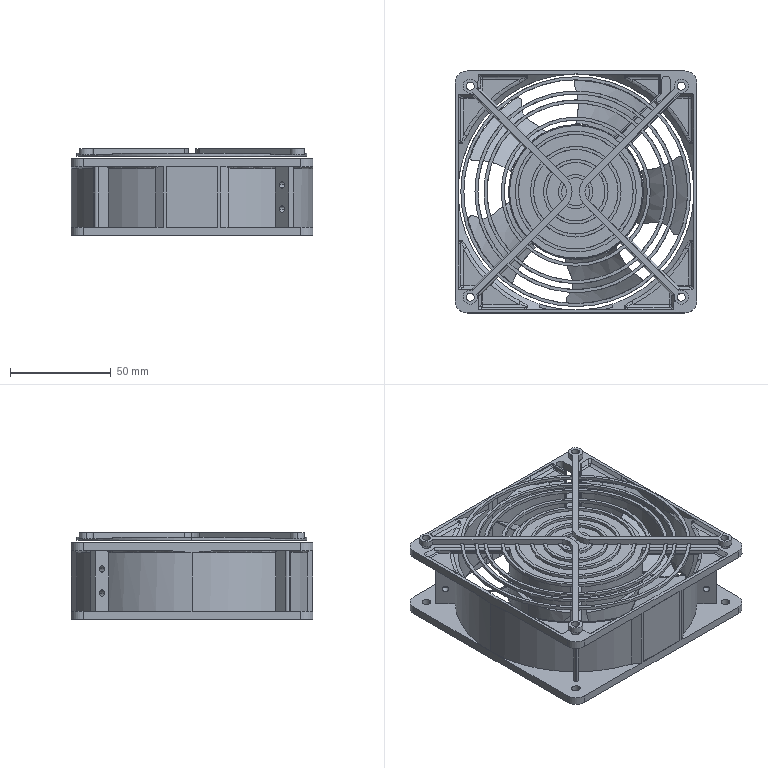Part | SolidWorks | features BaseBody 2 | 2 solids | 526 faces | box 120 x 120 x 43 mm | volume 168023 mm3 | plane 223 | cylinder 184 | spline 107 | cone 8 | torus 4 | commonest cylinder face diameters 2 x30 4 x16 4.3 x16 2.2 x12 7 x12 120 x9